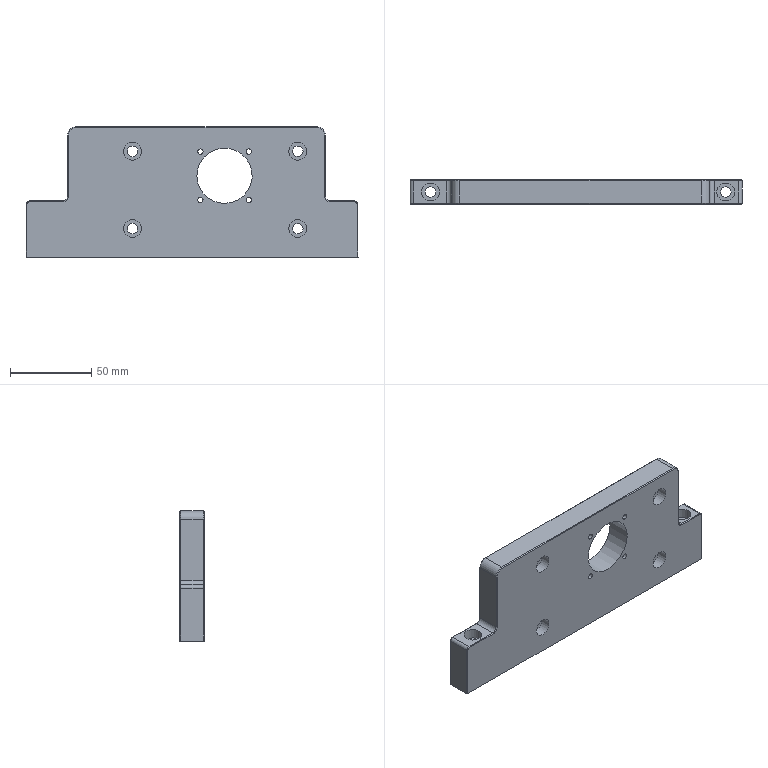Part | STEP file | ROTATION MC_NEW VER-0610_577 | 1 solid | 69 faces | box 204 x 15 x 80 mm | volume 192729 mm3 | plane 32 | cylinder 25 | cone 12 | commonest cylinder face diameters 6.5 x6 11 x6 3.3 x4 3.03 x2 4 x2 6 x2